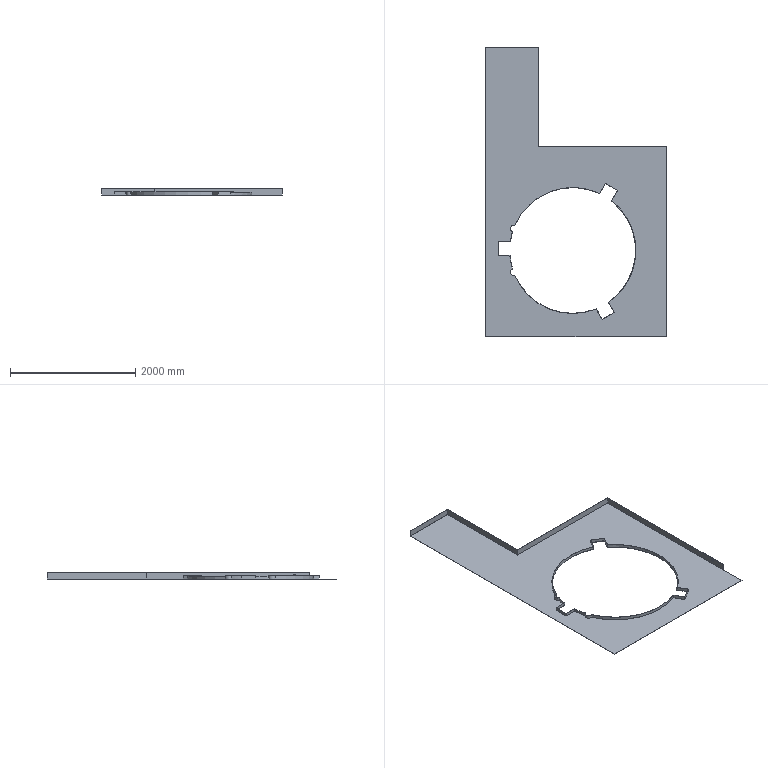Part | STEP file | PN_0024 third-floor left platform deck_Default<As Machined> | 7 solids | 113 faces | box 2885 x 4620 x 103 mm | volume 23616795 mm3 | plane 88 | cylinder 19 | torus 6 | commonest cylinder face diameters 2010 x7 2016 x5 100 x4 106 x2 35 x1